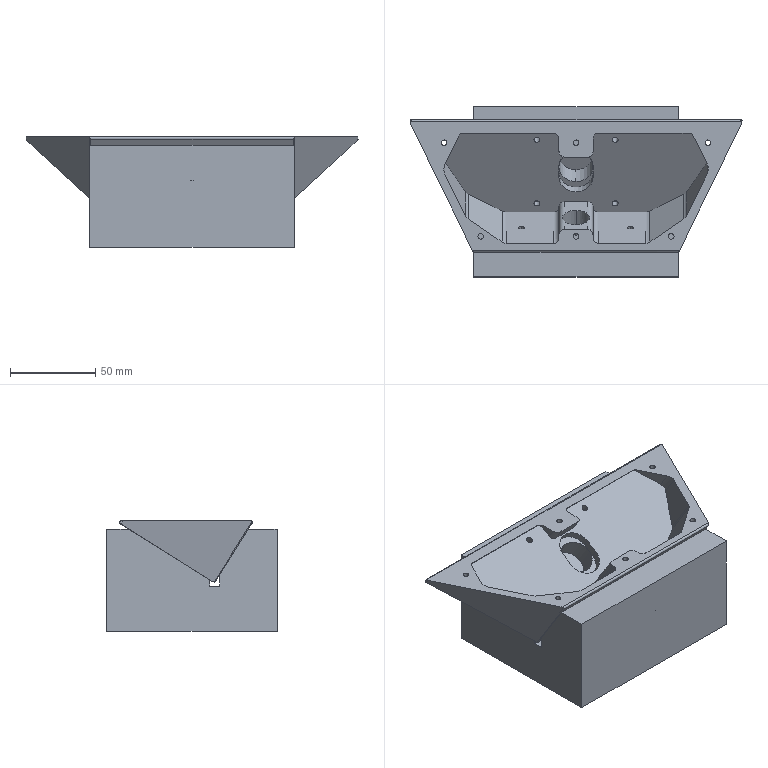NC program | Mastercam | posted with a generic post | part box 195.124 x 100 x 65 mm
Lines 1370 to 1918 of 1918:
N3780 T1 M6
N3790 G0 G90 G17 G55 X112.993 Y-25.632 A-32. S2300 M3
N3800 G43 H1 Z74.446
N3810 Z26.446
N3820 G1 Z24.146 F2000.
N3830 X-111.393 F3500.
N3840 G0 X-105.415 Y-14.967
N3850 G1 X105.415 F3500.
N3860 G0 X99.257 Y-4.302
N3870 G1 X-99.257 F3500.
N3880 G0 X-93.1 Y6.362
N3890 G1 X93.1 F3500.
N3900 G0 X86.943 Y17.027
N3910 G1 X-86.943 F3500.
N3920 G0 X-80.786 Y27.691
N3930 G1 X82.386 F3500.
N3940 Z23.846 F2000.
N3950 X-80.786 F3500.
N3960 G0 X-86.943 Y17.027
N3970 G1 X86.943 F3500.
N3980 G0 X93.1 Y6.362
N3990 G1 X-93.1 F3500.
N4000 G0 X-99.257 Y-4.302
N4010 G1 X99.257 F3500.
N4020 G0 X105.415 Y-14.967
N4030 G1 X-105.415 F3500.
N4040 G0 X-111.393 Y-25.632
N4050 G1 X112.993 F3500.
N4060 Z23.546 F2000.
N4070 X-111.393 F3500.
N4080 G0 X-105.415 Y-14.967
N4090 G1 X105.415 F3500.
N4100 G0 X99.257 Y-4.302
N4110 G1 X-99.257 F3500.
N4120 G0 X-93.1 Y6.362
N4130 G1 X93.1 F3500.
N4140 G0 X86.943 Y17.027
N4150 G1 X-86.943 F3500.
N4160 G0 X-80.786 Y27.691
N4170 G1 X82.386 F3500.
N4180 Z23.246 F2000.
N4190 X-80.786 F3500.
N4200 G0 X-86.943 Y17.027
N4210 G1 X86.943 F3500.
N4220 G0 X93.1 Y6.362
N4230 G1 X-93.1 F3500.
N4240 G0 X-99.257 Y-4.302
N4250 G1 X99.257 F3500.
N4260 G0 X105.415 Y-14.967
N4270 G1 X-105.415 F3500.
N4280 G0 X-111.393 Y-25.632
N4290 G1 X112.993 F3500.
N4300 Z22.946 F2000.
N4310 X-111.393 F3500.
N4320 G0 X-105.415 Y-14.967
N4330 G1 X105.415 F3500.
N4340 G0 X99.257 Y-4.302
N4350 G1 X-99.257 F3500.
N4360 G0 X-93.1 Y6.362
N4370 G1 X93.1 F3500.
N4380 G0 X86.943 Y17.027
N4390 G1 X-86.943 F3500.
N4400 G0 X-80.786 Y27.691
N4410 G1 X82.386 F3500.
N4420 Z22.646 F2000.
N4430 X-80.786 F3500.
N4440 G0 X-86.943 Y17.027
N4450 G1 X86.943 F3500.
N4460 G0 X93.1 Y6.362
N4470 G1 X-93.1 F3500.
N4480 G0 X-99.257 Y-4.302
N4490 G1 X99.257 F3500.
N4500 G0 X105.415 Y-14.967
N4510 G1 X-105.415 F3500.
N4520 G0 X-111.393 Y-25.632
N4530 G1 X112.993 F3500.
N4540 Z22.346 F2000.
N4550 X-111.393 F3500.
N4560 G0 X-105.415 Y-14.967
N4570 G1 X105.415 F3500.
N4580 G0 X99.257 Y-4.302
N4590 G1 X-99.257 F3500.
N4600 G0 X-93.1 Y6.362
N4610 G1 X93.1 F3500.
N4620 G0 X86.943 Y17.027
N4630 G1 X-86.943 F3500.
N4640 G0 X-80.786 Y27.691
N4650 G1 X82.386 F3500.
N4660 Z22.046 F2000.
N4670 X-80.786 F3500.
N4680 G0 X-86.943 Y17.027
N4690 G1 X86.943 F3500.
N4700 G0 X93.1 Y6.362
N4710 G1 X-93.1 F3500.
N4720 G0 X-99.257 Y-4.302
N4730 G1 X99.257 F3500.
N4740 G0 X105.415 Y-14.967
N4750 G1 X-105.415 F3500.
N4760 G0 X-111.393 Y-25.632
N4770 G1 X112.993 F3500.
N4780 G0 Z72.046
N4790 G56 X75.9 Y-15.944 Z86.193 A58.
N4800 Z38.193
N4810 G1 Z35.893 F2000.
N4820 X-74.3 F3500.
N4830 G0 Y-6.213
N4840 G1 X74.3 F3500.
N4850 G0 Y3.517
N4860 G1 X-74.3 F3500.
N4870 G0 Y13.248
N4880 G1 X75.9 F3500.
N4890 Z35.593 F2000.
N4900 X-74.3 F3500.
N4910 G0 Y3.517
N4920 G1 X74.3 F3500.
N4930 G0 Y-6.213
N4940 G1 X-74.3 F3500.
N4950 G0 Y-15.944
N4960 G1 X75.9 F3500.
N4970 Z35.293 F2000.
N4980 X-74.3 F3500.
N4990 G0 Y-6.213
N5000 G1 X74.3 F3500.
N5010 G0 Y3.517
N5020 G1 X-74.3 F3500.
N5030 G0 Y13.248
N5040 G1 X75.9 F3500.
N5050 Z34.993 F2000.
N5060 X-74.3 F3500.
N5070 G0 Y3.517
N5080 G1 X74.3 F3500.
N5090 G0 Y-6.213
N5100 G1 X-74.3 F3500.
N5110 G0 Y-15.944
N5120 G1 X75.9 F3500.
N5130 Z34.693 F2000.
N5140 X-74.3 F3500.
N5150 G0 Y-6.213
N5160 G1 X74.3 F3500.
N5170 G0 Y3.517
N5180 G1 X-74.3 F3500.
N5190 G0 Y13.248
N5200 G1 X75.9 F3500.
N5210 Z34.393 F2000.
N5220 X-74.3 F3500.
N5230 G0 Y3.517
N5240 G1 X74.3 F3500.
N5250 G0 Y-6.213
N5260 G1 X-74.3 F3500.
N5270 G0 Y-15.944
N5280 G1 X75.9 F3500.
N5290 Z34.093 F2000.
N5300 X-74.3 F3500.
N5310 G0 Y-6.213
N5320 G1 X74.3 F3500.
N5330 G0 Y3.517
N5340 G1 X-74.3 F3500.
N5350 G0 Y13.248
N5360 G1 X75.9 F3500.
N5370 Z33.793 F2000.
N5380 X-74.3 F3500.
N5390 G0 Y3.517
N5400 G1 X74.3 F3500.
N5410 G0 Y-6.213
N5420 G1 X-74.3 F3500.
N5430 G0 Y-15.944
N5440 G1 X75.9 F3500.
N5450 G0 Z83.793
N5460 G57 X92.276 Y-17.944 Z121.308 A58.
N5470 Z73.308
N5480 G1 Z71.008 F2000.
N5490 X-13.479 F3500.
N5500 G0 Y-6.548
N5510 G1 X83.343 F3500.
N5520 G0 X62.284 Y4.849
N5530 G1 X-13.479 F3500.
N5540 G0 Y16.245
N5550 G1 X42.824 F3500.
N5560 Z70.708 F2000.
N5570 X-13.479 F3500.
N5580 G0 Y4.849
N5590 G1 X62.284 F3500.
N5600 G0 X83.343 Y-6.548
N5610 G1 X-13.479 F3500.
N5620 G0 Y-17.944
N5630 G1 X92.276 F3500.
N5640 Z70.408 F2000.
N5650 X-13.479 F3500.
N5660 G0 Y-6.548
N5670 G1 X83.343 F3500.
N5680 G0 X62.284 Y4.849
N5690 G1 X-13.479 F3500.
N5700 G0 Y16.245
N5710 G1 X42.824 F3500.
N5720 Z70.108 F2000.
N5730 X-13.479 F3500.
N5740 G0 Y4.849
N5750 G1 X62.284 F3500.
N5760 G0 X83.343 Y-6.548
N5770 G1 X-13.479 F3500.
N5780 G0 Y-17.944
N5790 G1 X92.276 F3500.
N5800 Z69.808 F2000.
N5810 X-13.479 F3500.
N5820 G0 Y-6.548
N5830 G1 X83.343 F3500.
N5840 G0 X62.284 Y4.849
N5850 G1 X-13.479 F3500.
N5860 G0 Y16.245
N5870 G1 X42.824 F3500.
N5880 Z69.508 F2000.
N5890 X-13.479 F3500.
N5900 G0 Y4.849
N5910 G1 X62.284 F3500.
N5920 G0 X83.343 Y-6.548
N5930 G1 X-13.479 F3500.
N5940 G0 Y-17.944
N5950 G1 X92.276 F3500.
N5960 Z69.208 F2000.
N5970 X-13.479 F3500.
N5980 G0 Y-6.548
N5990 G1 X83.343 F3500.
N6000 G0 X62.284 Y4.849
N6010 G1 X-13.479 F3500.
N6020 G0 Y16.245
N6030 G1 X42.824 F3500.
N6040 Z68.908 F2000.
N6050 X-13.479 F3500.
N6060 G0 Y4.849
N6070 G1 X62.284 F3500.
N6080 G0 X83.343 Y-6.548
N6090 G1 X-13.479 F3500.
N6100 G0 Y-17.944
N6110 G1 X92.276 F3500.
N6120 G0 Z118.908
N6130 G58 X12.079 Y-17.944 Z121.308 A58.
N6140 Z73.308
N6150 G1 Z71.008 F2000.
N6160 X-87.676 F3500.
N6170 G0 X-77.04 Y-6.548
N6180 G1 X10.479 F3500.
N6190 G0 Y4.849
N6200 G1 X-55.98 F3500.
N6210 G0 X-34.921 Y16.245
N6220 G1 X12.079 F3500.
N6230 Z70.708 F2000.
N6240 X-34.921 F3500.
N6250 G0 X-55.98 Y4.849
N6260 G1 X10.479 F3500.
N6270 G0 Y-6.548
N6280 G1 X-77.04 F3500.
N6290 G0 X-87.676 Y-17.944
N6300 G1 X12.079 F3500.
N6310 Z70.408 F2000.
N6320 X-87.676 F3500.
N6330 G0 X-77.04 Y-6.548
N6340 G1 X10.479 F3500.
N6350 G0 Y4.849
N6360 G1 X-55.98 F3500.
N6370 G0 X-34.921 Y16.245
N6380 G1 X12.079 F3500.
N6390 Z70.108 F2000.
N6400 X-34.921 F3500.
N6410 G0 X-55.98 Y4.849
N6420 G1 X10.479 F3500.
N6430 G0 Y-6.548
N6440 G1 X-77.04 F3500.
N6450 G0 X-87.676 Y-17.944
N6460 G1 X12.079 F3500.
N6470 Z69.808 F2000.
N6480 X-87.676 F3500.
N6490 G0 X-77.04 Y-6.548
N6500 G1 X10.479 F3500.
N6510 G0 Y4.849
N6520 G1 X-55.98 F3500.
N6530 G0 X-34.921 Y16.245
N6540 G1 X12.079 F3500.
N6550 Z69.508 F2000.
N6560 X-34.921 F3500.
N6570 G0 X-55.98 Y4.849
N6580 G1 X10.479 F3500.
N6590 G0 Y-6.548
N6600 G1 X-77.04 F3500.
N6610 G0 X-87.676 Y-17.944
N6620 G1 X12.079 F3500.
N6630 Z69.208 F2000.
N6640 X-87.676 F3500.
N6650 G0 X-77.04 Y-6.548
N6660 G1 X10.479 F3500.
N6670 G0 Y4.849
N6680 G1 X-55.98 F3500.
N6690 G0 X-34.921 Y16.245
N6700 G1 X12.079 F3500.
N6710 Z68.908 F2000.
N6720 X-34.921 F3500.
N6730 G0 X-55.98 Y4.849
N6740 G1 X10.479 F3500.
N6750 G0 Y-6.548
N6760 G1 X-77.04 F3500.
N6770 G0 X-87.676 Y-17.944
N6780 G1 X12.079 F3500.
N6790 G0 Z118.908
N6800 G59 X47.97 Y13.25 Z111.329 A58.
N6810 Z62.329
N6820 G1 Z61.029 F2000.
N6830 G41 D1 X41.97 F3500.
N6840 X36.509
N6850 Y-15.946
N6860 X42.284
N6870 G40 X48.284
N6880 Z60.729 F2000.
N6890 G42 D1 X42.284 F3500.
N6900 X36.509
N6910 Y13.25
N6920 X41.97
N6930 G40 X47.97
N6940 Z60.429 F2000.
N6950 G41 D1 X41.97 F3500.
N6960 X36.509
N6970 Y-15.946
N6980 X42.284
N6990 G40 X48.284
N7000 Z60.129 F2000.
N7010 G42 D1 X42.284 F3500.
N7020 X36.509
N7030 Y13.25
N7040 X41.97
N7050 G40 X47.97
N7060 Z59.829 F2000.
N7070 G41 D1 X41.97 F3500.
N7080 X36.509
N7090 Y-15.946
N7100 X42.284
N7110 G40 X48.284
N7120 Z59.529 F2000.
N7130 G42 D1 X42.284 F3500.
N7140 X36.509
N7150 Y13.25
N7160 X41.97
N7170 G40 X47.97
N7180 Z59.229 F2000.
N7190 G41 D1 X41.97 F3500.
N7200 X36.509
N7210 Y-15.946
N7220 X42.284
N7230 G40 X48.284
N7240 Z58.929 F2000.
N7250 G42 D1 X42.284 F3500.
N7260 X36.509
N7270 Y13.25
N7280 X41.97
N7290 G40 X47.97
N7300 G0 Z111.329
N7310 G54.1 P1 X-48.284 Y-15.946 Z111.329 A58.
N7320 Z62.329
N7330 G1 Z61.029 F2000.
N7340 G41 D1 X-42.284 F3500.
N7350 X-36.509
N7360 Y13.25
N7370 X-41.97
N7380 G40 X-47.97
N7390 Z60.729 F2000.
N7400 G42 D1 X-41.97 F3500.
N7410 X-36.509
N7420 Y-15.946
N7430 X-42.284
N7440 G40 X-48.284
N7450 Z60.429 F2000.
N7460 G41 D1 X-42.284 F3500.
N7470 X-36.509
N7480 Y13.25
N7490 X-41.97
N7500 G40 X-47.97
N7510 Z60.129 F2000.
N7520 G42 D1 X-41.97 F3500.
N7530 X-36.509
N7540 Y-15.946
N7550 X-42.284
N7560 G40 X-48.284
N7570 Z59.829 F2000.
N7580 G41 D1 X-42.284 F3500.
N7590 X-36.509
N7600 Y13.25
N7610 X-41.97
N7620 G40 X-47.97
N7630 Z59.529 F2000.
N7640 G42 D1 X-41.97 F3500.
N7650 X-36.509
N7660 Y-15.946
N7670 X-42.284
N7680 G40 X-48.284
N7690 Z59.229 F2000.
N7700 G41 D1 X-42.284 F3500.
N7710 X-36.509
N7720 Y13.25
N7730 X-41.97
N7740 G40 X-47.97
N7750 Z58.929 F2000.
N7760 G42 D1 X-41.97 F3500.
N7770 X-36.509
N7780 Y-15.946
N7790 X-42.284
N7800 G40 X-48.284
N7810 G0 Z111.329
N7820 M5
N7830 G91 G28 Z0.
N7840 A0.
N7850 M01
N7860 T2 M6
N7870 G0 G90 G17 G55 X112.993 Y-25.632 A-32. S4500 M3
N7880 G43 H2 Z74.446
N7890 Z26.446
N7900 G1 Z21.946 F2000.
N7910 X-111.393 F600.
N7920 G0 X-105.415 Y-14.967
N7930 G1 X105.415 F600.
N7940 G0 X99.257 Y-4.302
N7950 G1 X-99.257 F600.
N7960 G0 X-93.1 Y6.362
N7970 G1 X93.1 F600.
N7980 G0 X86.943 Y17.027
N7990 G1 X-86.943 F600.
N8000 G0 X-80.786 Y27.691
N8010 G1 X82.386 F600.
N8020 G0 Z71.946
N8030 G56 X75.9 Y-15.944 Z86.193 A58.
N8040 Z38.193
N8050 G1 Z33.693 F2000.
N8060 X-74.3 F600.
N8070 G0 Y-6.213
N8080 G1 X74.3 F600.
N8090 G0 Y3.517
N8100 G1 X-74.3 F600.
N8110 G0 Y13.248
N8120 G1 X75.9 F600.
N8130 G0 Z83.693
N8140 G57 X92.276 Y-17.944 Z121.308 A58.
N8150 Z73.308
N8160 G1 Z68.808 F2000.
N8170 X-13.479 F600.
N8180 G0 Y-6.548
N8190 G1 X83.343 F600.
N8200 G0 X62.284 Y4.849
N8210 G1 X-13.479 F600.
N8220 G0 Y16.245
N8230 G1 X42.824 F600.
N8240 G0 Z118.808
N8250 G58 X12.079 Y-17.944 Z121.308 A58.
N8260 Z73.308
N8270 G1 Z68.808 F2000.
N8280 X-87.676 F600.
N8290 G0 X-77.04 Y-6.548
N8300 G1 X10.479 F600.
N8310 G0 Y4.849
N8320 G1 X-55.98 F600.
N8330 G0 X-34.921 Y16.245
N8340 G1 X12.079 F600.
N8350 G0 Z118.808
N8360 G59 X47.97 Y13.25 Z91.329 A58.
N8370 Z62.329
N8380 G1 Z58.829 F2000.
N8390 G41 D2 X41.97 F600.
N8400 X36.509
N8410 Y-15.946
N8420 X42.284
N8430 G40 X48.284
N8440 G0 Z91.329
N8450 G54.1 P1 X-48.284 Y-15.946 Z91.329 A58.
N8460 Z62.329
N8470 G1 Z58.829 F2000.
N8480 G41 D2 X-42.284 F600.
N8490 X-36.509
N8500 Y13.25
N8510 X-41.97
N8520 G40 X-47.97
N8530 G0 Z91.329
N8540 M5
N8550 G91 G28 Z0.
N8560 A0.
N8570 M01
N8580 T3 M6
N8590 G0 G90 G17 G55 X-22.959 Y-21.307 A-32. S2000 M3
N8600 G43 H3 Z51.946
N8610 G98 G81 Z20.196 R22.946 F100.
N8620 Y22.693
N8630 X23.041
N8640 Y-21.307
N8650 G80
N8660 G56 X-32. Y.554 Z63.693 A58.
N8670 G0
N8680 G98 G81 Z31.693 R34.693 F100.
N8690 X32.
N8700 G80
N8710 M5
N8720 G91 G0 G28 Z0.
N8730 A0.
N8740 M01
N8750 T4 M6
N8760 G0 G90 G17 G56 X-32. Y.554 A58. S1200 M3
N8770 G43 H4 Z63.693
N8780 G98 G81 Z25.693 R34.693 F100.
N8790 X32.
N8800 G80
N8810 M5
N8820 G91 G0 G28 Z0.
N8830 A0.
N8840 M01
N8850 T5 M6
N8860 G0 G90 G17 G56 X-32. Y.554 A58. S300 M3
N8870 G43 H5 Z63.693
N8880 G94
N8890 G98 G84 Z25.693 R34.693 F210.
N8900 X32.
N8910 G80
N8920 G94
N8930 M5
N8940 G91 G0 G28 Z0.
N8950 A0.
N8960 M01
N8970 T11 M6
N8980 G0 G90 G17 G55 X-22.959 Y-21.307 A-32. S1200 M3
N8990 G43 H11 Z51.946
N9000 G98 G81 Z13.946 R22.946 F100.
N9010 Y22.693
N9020 X23.041
N9030 Y-21.307
N9040 G80
N9050 M5
N9060 G91 G0 G28 Z0.
N9070 A0.
N9080 M01
N9090 T7 M6
N9100 G0 G90 G17 G55 X-99.419 Y-32.582 A-32. S3500 M3
N9110 G43 H7 Z54.446
N9120 Z25.446
N9130 G1 Z20.746 F2000.
N9140 G41 D7 X-98.294 Y-30.634 F800.
N9150 X-61.082 Y33.819
N9160 X-59.568 Y34.693
N9170 X59.568
N9180 X61.082 Y33.819
N9190 X98.294 Y-30.634
N9200 G40 X99.419 Y-32.582
N9210 G0 Z54.446
N9220 M5
N9230 G91 G28 Z0.
N9240 G28 X0. Y0. A0.
N9250 M30
%